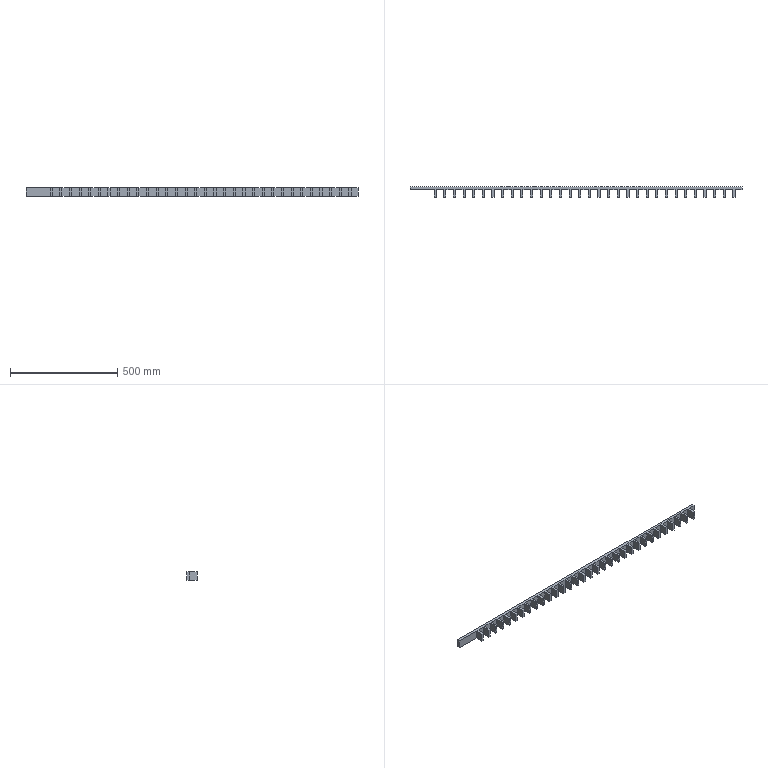Part | SolidWorks | features ICE 8, MoveFace 2, Extrusion 1 | 1 solid | 134 faces | box 1550 x 48 x 40 mm | volume 1254000 mm3 | plane 134